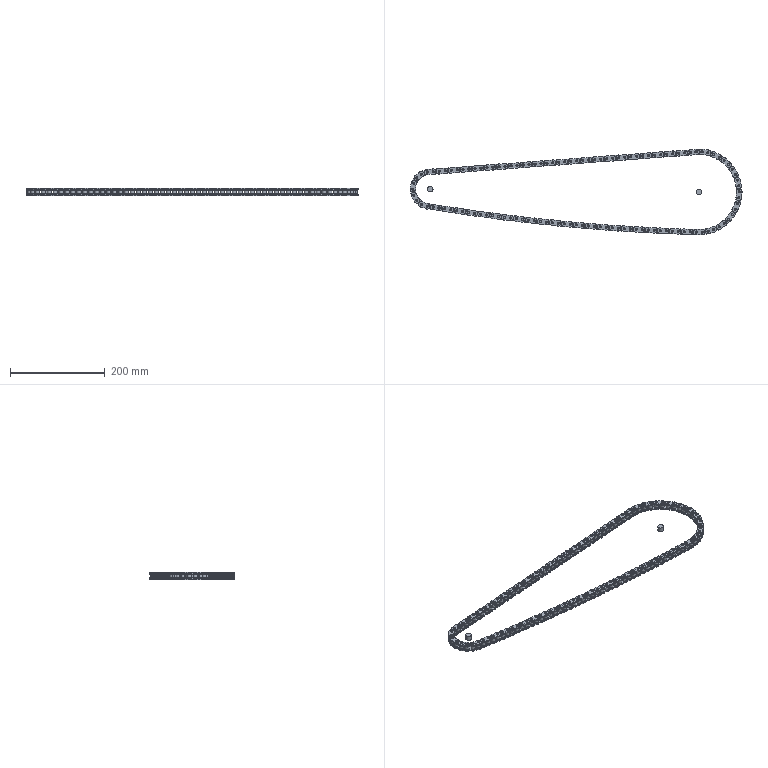Part | SolidWorks | features BaseBody 182 | 182 solids | 3608 faces | volume 164933 mm3 | cylinder 2404 | plane 724 | cone 480 | commonest cylinder face diameters 4.45 x960 11.81 x720 57.066 x480 8.51 x240 12 x4